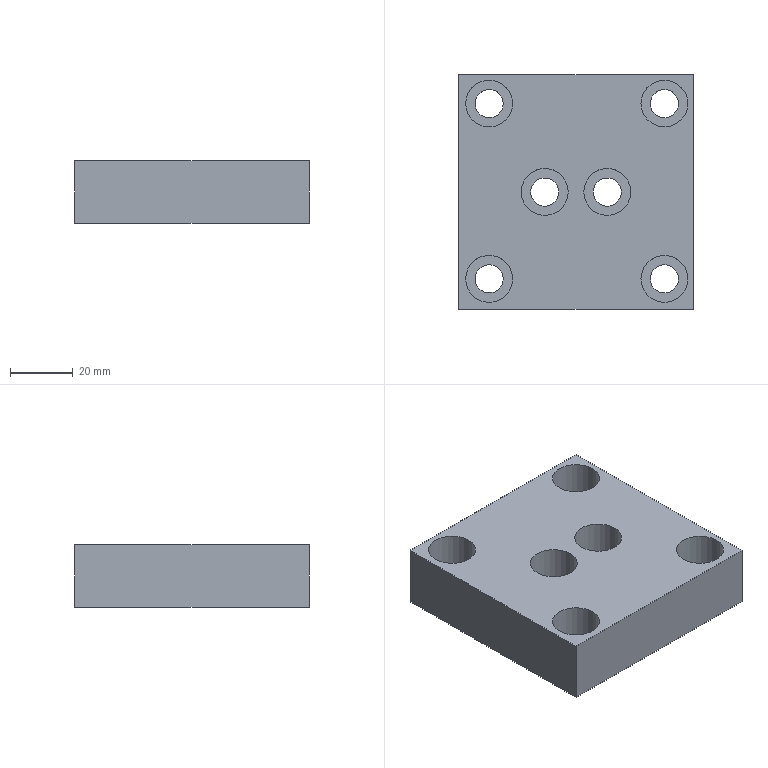Part | NX | features solid 2 | 1 solid | 24 faces | box 75 x 75 x 20 mm | volume 96271 mm3 | plane 12 | cylinder 12 | commonest cylinder face diameters 9 x6 15 x6
STEP:
#1=CARTESIAN_POINT('',(577.5,-142.5,340.));
#2=VERTEX_POINT('',#1);
#3=CARTESIAN_POINT('',(652.5,-142.5,340.));
#4=VERTEX_POINT('',#3);
#5=CARTESIAN_POINT('',(577.5,-142.5,340.));
#6=DIRECTION('',(1.,0.,0.));
#7=VECTOR('',#6,1000.);
#8=LINE('',#5,#7);
#9=EDGE_CURVE('',#2,#4,#8,.T.);
#10=ORIENTED_EDGE('',*,*,#9,.T.);
#11=CARTESIAN_POINT('',(652.5,-142.5,320.));
#12=VERTEX_POINT('',#11);
#13=CARTESIAN_POINT('',(652.5,-142.5,320.));
#14=DIRECTION('',(0.,0.,1.));
#15=VECTOR('',#14,1000.);
#16=LINE('',#13,#15);
#17=EDGE_CURVE('',#12,#4,#16,.T.);
#18=ORIENTED_EDGE('',*,*,#17,.F.);
#19=CARTESIAN_POINT('',(577.5,-142.5,320.));
#20=VERTEX_POINT('',#19);
#21=CARTESIAN_POINT('',(577.5,-142.5,320.));
#22=DIRECTION('',(1.,0.,0.));
#23=VECTOR('',#22,1000.);
#24=LINE('',#21,#23);
#25=EDGE_CURVE('',#20,#12,#24,.T.);
#26=ORIENTED_EDGE('',*,*,#25,.F.);
#27=CARTESIAN_POINT('',(577.5,-142.5,320.));
#28=DIRECTION('',(0.,0.,1.));
#29=VECTOR('',#28,1000.);
#30=LINE('',#27,#29);
#31=EDGE_CURVE('',#20,#2,#30,.T.);
#32=ORIENTED_EDGE('',*,*,#31,.T.);
#33=EDGE_LOOP('',(#10,#18,#26,#32));
#34=FACE_BOUND('',#33,.T.);
#35=CARTESIAN_POINT('',(577.5,-142.5,320.));
#36=DIRECTION('',(0.,-1.,0.));
#37=DIRECTION('',(0.,0.,-1.));
#38=AXIS2_PLACEMENT_3D('',#35,#36,#37);
#39=PLANE('',#38);
#40=ADVANCED_FACE('',(#34),#39,.F.);
#41=CARTESIAN_POINT('',(652.5,-217.5,340.));
#42=VERTEX_POINT('',#41);
#43=CARTESIAN_POINT('',(652.5,-217.5,340.));
#44=DIRECTION('',(0.,1.,0.));
#45=VECTOR('',#44,1000.);
#46=LINE('',#43,#45);
#47=EDGE_CURVE('',#42,#4,#46,.T.);
#48=ORIENTED_EDGE('',*,*,#47,.F.);
#49=CARTESIAN_POINT('',(652.5,-217.5,320.));
#50=VERTEX_POINT('',#49);
#51=CARTESIAN_POINT('',(652.5,-217.5,320.));
#52=DIRECTION('',(0.,0.,1.));
#53=VECTOR('',#52,1000.);
#54=LINE('',#51,#53);
#55=EDGE_CURVE('',#50,#42,#54,.T.);
#56=ORIENTED_EDGE('',*,*,#55,.F.);
#57=CARTESIAN_POINT('',(652.5,-217.5,320.));
#58=DIRECTION('',(0.,1.,0.));
#59=VECTOR('',#58,1000.);
#60=LINE('',#57,#59);
#61=EDGE_CURVE('',#50,#12,#60,.T.);
#62=ORIENTED_EDGE('',*,*,#61,.T.);
#63=ORIENTED_EDGE('',*,*,#17,.T.);
#64=EDGE_LOOP('',(#48,#56,#62,#63));
#65=FACE_BOUND('',#64,.T.);
#66=CARTESIAN_POINT('',(652.5,-217.5,320.));
#67=DIRECTION('',(1.,0.,0.));
#68=DIRECTION('',(0.,0.,-1.));
#69=AXIS2_PLACEMENT_3D('',#66,#67,#68);
#70=PLANE('',#69);
#71=ADVANCED_FACE('',(#65),#70,.T.);
#72=CARTESIAN_POINT('',(577.5,-217.5,340.));
#73=VERTEX_POINT('',#72);
#74=CARTESIAN_POINT('',(577.5,-217.5,340.));
#75=DIRECTION('',(1.,0.,0.));
#76=VECTOR('',#75,1000.);
#77=LINE('',#74,#76);
#78=EDGE_CURVE('',#73,#42,#77,.T.);
#79=ORIENTED_EDGE('',*,*,#78,.F.);
#80=CARTESIAN_POINT('',(577.5,-217.5,320.));
#81=VERTEX_POINT('',#80);
#82=CARTESIAN_POINT('',(577.5,-217.5,320.));
#83=DIRECTION('',(0.,0.,1.));
#84=VECTOR('',#83,1000.);
#85=LINE('',#82,#84);
#86=EDGE_CURVE('',#81,#73,#85,.T.);
#87=ORIENTED_EDGE('',*,*,#86,.F.);
#88=CARTESIAN_POINT('',(577.5,-217.5,320.));
#89=DIRECTION('',(1.,0.,0.));
#90=VECTOR('',#89,1000.);
#91=LINE('',#88,#90);
#92=EDGE_CURVE('',#81,#50,#91,.T.);
#93=ORIENTED_EDGE('',*,*,#92,.T.);
#94=ORIENTED_EDGE('',*,*,#55,.T.);
#95=EDGE_LOOP('',(#79,#87,#93,#94));
#96=FACE_BOUND('',#95,.T.);
#97=CARTESIAN_POINT('',(577.5,-217.5,320.));
#98=DIRECTION('',(0.,-1.,0.));
#99=DIRECTION('',(0.,0.,-1.));
#100=AXIS2_PLACEMENT_3D('',#97,#98,#99);
#101=PLANE('',#100);
#102=ADVANCED_FACE('',(#96),#101,.T.);
#103=CARTESIAN_POINT('',(577.5,-217.5,340.));
#104=DIRECTION('',(0.,1.,0.));
#105=VECTOR('',#104,1000.);
#106=LINE('',#103,#105);
#107=EDGE_CURVE('',#73,#2,#106,.T.);
#108=ORIENTED_EDGE('',*,*,#107,.T.);
#109=ORIENTED_EDGE('',*,*,#31,.F.);
#110=CARTESIAN_POINT('',(577.5,-217.5,320.));
#111=DIRECTION('',(0.,1.,0.));
#112=VECTOR('',#111,1000.);
#113=LINE('',#110,#112);
#114=EDGE_CURVE('',#81,#20,#113,.T.);
#115=ORIENTED_EDGE('',*,*,#114,.F.);
#116=ORIENTED_EDGE('',*,*,#86,.T.);
#117=EDGE_LOOP('',(#108,#109,#115,#116));
#118=FACE_BOUND('',#117,.T.);
#119=CARTESIAN_POINT('',(577.5,-217.5,320.));
#120=DIRECTION('',(1.,0.,0.));
#121=DIRECTION('',(0.,0.,-1.));
#122=AXIS2_PLACEMENT_3D('',#119,#120,#121);
#123=PLANE('',#122);
#124=ADVANCED_FACE('',(#118),#123,.F.);
#125=CARTESIAN_POINT('',(638.75,-207.75,320.));
#126=VERTEX_POINT('',#125);
#127=CARTESIAN_POINT('',(643.25,-207.75,320.));
#128=DIRECTION('',(0.,0.,-1.));
#129=DIRECTION('',(-1.,0.,0.));
#130=AXIS2_PLACEMENT_3D('',#127,#128,#129);
#131=CIRCLE('',#130,4.5);
#132=EDGE_CURVE('',#126,#126,#131,.T.);
#133=ORIENTED_EDGE('',*,*,#132,.F.);
#134=EDGE_LOOP('',(#133));
#135=FACE_BOUND('',#134,.T.);
#136=CARTESIAN_POINT('',(582.75,-207.75,320.));
#137=VERTEX_POINT('',#136);
#138=CARTESIAN_POINT('',(587.25,-207.75,320.));
#139=DIRECTION('',(0.,0.,-1.));
#140=DIRECTION('',(-1.,0.,0.));
#141=AXIS2_PLACEMENT_3D('',#138,#139,#140);
#142=CIRCLE('',#141,4.5);
#143=EDGE_CURVE('',#137,#137,#142,.T.);
#144=ORIENTED_EDGE('',*,*,#143,.F.);
#145=EDGE_LOOP('',(#144));
#146=FACE_BOUND('',#145,.T.);
#147=CARTESIAN_POINT('',(582.75,-151.75,320.));
#148=VERTEX_POINT('',#147);
#149=CARTESIAN_POINT('',(587.25,-151.75,320.));
#150=DIRECTION('',(0.,0.,-1.));
#151=DIRECTION('',(-1.,0.,0.));
#152=AXIS2_PLACEMENT_3D('',#149,#150,#151);
#153=CIRCLE('',#152,4.5);
#154=EDGE_CURVE('',#148,#148,#153,.T.);
#155=ORIENTED_EDGE('',*,*,#154,.F.);
#156=EDGE_LOOP('',(#155));
#157=FACE_BOUND('',#156,.T.);
#158=CARTESIAN_POINT('',(638.75,-151.75,320.));
#159=VERTEX_POINT('',#158);
#160=CARTESIAN_POINT('',(643.25,-151.75,320.));
#161=DIRECTION('',(0.,0.,-1.));
#162=DIRECTION('',(-1.,0.,0.));
#163=AXIS2_PLACEMENT_3D('',#160,#161,#162);
#164=CIRCLE('',#163,4.5);
#165=EDGE_CURVE('',#159,#159,#164,.T.);
#166=ORIENTED_EDGE('',*,*,#165,.F.);
#167=EDGE_LOOP('',(#166));
#168=FACE_BOUND('',#167,.T.);
#169=CARTESIAN_POINT('',(600.5,-180.,320.));
#170=VERTEX_POINT('',#169);
#171=CARTESIAN_POINT('',(605.,-180.,320.));
#172=DIRECTION('',(0.,0.,-1.));
#173=DIRECTION('',(-1.,0.,0.));
#174=AXIS2_PLACEMENT_3D('',#171,#172,#173);
#175=CIRCLE('',#174,4.5);
#176=EDGE_CURVE('',#170,#170,#175,.T.);
#177=ORIENTED_EDGE('',*,*,#176,.F.);
#178=EDGE_LOOP('',(#177));
#179=FACE_BOUND('',#178,.T.);
#180=CARTESIAN_POINT('',(620.5,-180.,320.));
#181=VERTEX_POINT('',#180);
#182=CARTESIAN_POINT('',(625.,-180.,320.));
#183=DIRECTION('',(0.,0.,-1.));
#184=DIRECTION('',(-1.,0.,0.));
#185=AXIS2_PLACEMENT_3D('',#182,#183,#184);
#186=CIRCLE('',#185,4.5);
#187=EDGE_CURVE('',#181,#181,#186,.T.);
#188=ORIENTED_EDGE('',*,*,#187,.F.);
#189=EDGE_LOOP('',(#188));
#190=FACE_BOUND('',#189,.T.);
#191=ORIENTED_EDGE('',*,*,#25,.T.);
#192=ORIENTED_EDGE('',*,*,#61,.F.);
#193=ORIENTED_EDGE('',*,*,#92,.F.);
#194=ORIENTED_EDGE('',*,*,#114,.T.);
#195=EDGE_LOOP('',(#191,#192,#193,#194));
#196=FACE_BOUND('',#195,.T.);
#197=CARTESIAN_POINT('',(652.5,-142.5,320.));
#198=DIRECTION('',(0.,0.,1.));
#199=DIRECTION('',(1.,0.,0.));
#200=AXIS2_PLACEMENT_3D('',#197,#198,#199);
#201=PLANE('',#200);
#202=ADVANCED_FACE('',(#135,#146,#157,#168,#179,#190,#196),#201,.F.);
#203=CARTESIAN_POINT('',(635.75,-207.75,340.));
#204=VERTEX_POINT('',#203);
#205=CARTESIAN_POINT('',(643.25,-207.75,340.));
#206=DIRECTION('',(0.,0.,-1.));
#207=DIRECTION('',(-1.,0.,0.));
#208=AXIS2_PLACEMENT_3D('',#205,#206,#207);
#209=CIRCLE('',#208,7.5);
#210=EDGE_CURVE('',#204,#204,#209,.T.);
#211=ORIENTED_EDGE('',*,*,#210,.T.);
#212=EDGE_LOOP('',(#211));
#213=FACE_BOUND('',#212,.T.);
#214=CARTESIAN_POINT('',(579.75,-207.75,340.));
#215=VERTEX_POINT('',#214);
#216=CARTESIAN_POINT('',(587.25,-207.75,340.));
#217=DIRECTION('',(0.,0.,-1.));
#218=DIRECTION('',(-1.,0.,0.));
#219=AXIS2_PLACEMENT_3D('',#216,#217,#218);
#220=CIRCLE('',#219,7.5);
#221=EDGE_CURVE('',#215,#215,#220,.T.);
#222=ORIENTED_EDGE('',*,*,#221,.T.);
#223=EDGE_LOOP('',(#222));
#224=FACE_BOUND('',#223,.T.);
#225=CARTESIAN_POINT('',(579.75,-151.75,340.));
#226=VERTEX_POINT('',#225);
#227=CARTESIAN_POINT('',(587.25,-151.75,340.));
#228=DIRECTION('',(0.,0.,-1.));
#229=DIRECTION('',(-1.,0.,0.));
#230=AXIS2_PLACEMENT_3D('',#227,#228,#229);
#231=CIRCLE('',#230,7.5);
#232=EDGE_CURVE('',#226,#226,#231,.T.);
#233=ORIENTED_EDGE('',*,*,#232,.T.);
#234=EDGE_LOOP('',(#233));
#235=FACE_BOUND('',#234,.T.);
#236=CARTESIAN_POINT('',(635.75,-151.75,340.));
#237=VERTEX_POINT('',#236);
#238=CARTESIAN_POINT('',(643.25,-151.75,340.));
#239=DIRECTION('',(0.,0.,-1.));
#240=DIRECTION('',(-1.,0.,0.));
#241=AXIS2_PLACEMENT_3D('',#238,#239,#240);
#242=CIRCLE('',#241,7.5);
#243=EDGE_CURVE('',#237,#237,#242,.T.);
#244=ORIENTED_EDGE('',*,*,#243,.T.);
#245=EDGE_LOOP('',(#244));
#246=FACE_BOUND('',#245,.T.);
#247=CARTESIAN_POINT('',(597.5,-180.,340.));
#248=VERTEX_POINT('',#247);
#249=CARTESIAN_POINT('',(605.,-180.,340.));
#250=DIRECTION('',(0.,0.,-1.));
#251=DIRECTION('',(-1.,0.,0.));
#252=AXIS2_PLACEMENT_3D('',#249,#250,#251);
#253=CIRCLE('',#252,7.5);
#254=EDGE_CURVE('',#248,#248,#253,.T.);
#255=ORIENTED_EDGE('',*,*,#254,.T.);
#256=EDGE_LOOP('',(#255));
#257=FACE_BOUND('',#256,.T.);
#258=CARTESIAN_POINT('',(617.5,-180.,340.));
#259=VERTEX_POINT('',#258);
#260=CARTESIAN_POINT('',(625.,-180.,340.));
#261=DIRECTION('',(0.,0.,-1.));
#262=DIRECTION('',(-1.,0.,0.));
#263=AXIS2_PLACEMENT_3D('',#260,#261,#262);
#264=CIRCLE('',#263,7.5);
#265=EDGE_CURVE('',#259,#259,#264,.T.);
#266=ORIENTED_EDGE('',*,*,#265,.T.);
#267=EDGE_LOOP('',(#266));
#268=FACE_BOUND('',#267,.T.);
#269=ORIENTED_EDGE('',*,*,#9,.F.);
#270=ORIENTED_EDGE('',*,*,#107,.F.);
#271=ORIENTED_EDGE('',*,*,#78,.T.);
#272=ORIENTED_EDGE('',*,*,#47,.T.);
#273=EDGE_LOOP('',(#269,#270,#271,#272));
#274=FACE_BOUND('',#273,.T.);
#275=CARTESIAN_POINT('',(652.5,-142.5,340.));
#276=DIRECTION('',(0.,0.,1.));
#277=DIRECTION('',(1.,0.,0.));
#278=AXIS2_PLACEMENT_3D('',#275,#276,#277);
#279=PLANE('',#278);
#280=ADVANCED_FACE('',(#213,#224,#235,#246,#257,#268,#274),#279,.T.);
#281=ORIENTED_EDGE('',*,*,#187,.T.);
#282=EDGE_LOOP('',(#281));
#283=FACE_BOUND('',#282,.T.);
#284=CARTESIAN_POINT('',(620.5,-180.,326.));
#285=VERTEX_POINT('',#284);
#286=CARTESIAN_POINT('',(625.,-180.,326.));
#287=DIRECTION('',(0.,0.,-1.));
#288=DIRECTION('',(-1.,0.,0.));
#289=AXIS2_PLACEMENT_3D('',#286,#287,#288);
#290=CIRCLE('',#289,4.5);
#291=EDGE_CURVE('',#285,#285,#290,.T.);
#292=ORIENTED_EDGE('',*,*,#291,.F.);
#293=EDGE_LOOP('',(#292));
#294=FACE_BOUND('',#293,.T.);
#295=CARTESIAN_POINT('',(625.,-180.,320.));
#296=DIRECTION('',(0.,0.,-1.));
#297=DIRECTION('',(-1.,0.,0.));
#298=AXIS2_PLACEMENT_3D('',#295,#296,#297);
#299=CYLINDRICAL_SURFACE('',#298,4.5);
#300=ADVANCED_FACE('',(#283,#294),#299,.F.);
#301=ORIENTED_EDGE('',*,*,#291,.T.);
#302=EDGE_LOOP('',(#301));
#303=FACE_BOUND('',#302,.T.);
#304=CARTESIAN_POINT('',(617.5,-180.,326.));
#305=VERTEX_POINT('',#304);
#306=CARTESIAN_POINT('',(625.,-180.,326.));
#307=DIRECTION('',(0.,0.,-1.));
#308=DIRECTION('',(-1.,0.,0.));
#309=AXIS2_PLACEMENT_3D('',#306,#307,#308);
#310=CIRCLE('',#309,7.5);
#311=EDGE_CURVE('',#305,#305,#310,.T.);
#312=ORIENTED_EDGE('',*,*,#311,.F.);
#313=EDGE_LOOP('',(#312));
#314=FACE_BOUND('',#313,.T.);
#315=CARTESIAN_POINT('',(625.,-180.,326.));
#316=DIRECTION('',(0.,0.,-1.));
#317=DIRECTION('',(-1.,0.,0.));
#318=AXIS2_PLACEMENT_3D('',#315,#316,#317);
#319=PLANE('',#318);
#320=ADVANCED_FACE('',(#303,#314),#319,.F.);
#321=ORIENTED_EDGE('',*,*,#311,.T.);
#322=EDGE_LOOP('',(#321));
#323=FACE_BOUND('',#322,.T.);
#324=ORIENTED_EDGE('',*,*,#265,.F.);
#325=EDGE_LOOP('',(#324));
#326=FACE_BOUND('',#325,.T.);
#327=CARTESIAN_POINT('',(625.,-180.,340.));
#328=DIRECTION('',(0.,0.,-1.));
#329=DIRECTION('',(-1.,0.,0.));
#330=AXIS2_PLACEMENT_3D('',#327,#328,#329);
#331=CYLINDRICAL_SURFACE('',#330,7.5);
#332=ADVANCED_FACE('',(#323,#326),#331,.F.);
#333=ORIENTED_EDGE('',*,*,#176,.T.);
#334=EDGE_LOOP('',(#333));
#335=FACE_BOUND('',#334,.T.);
#336=CARTESIAN_POINT('',(600.5,-180.,326.));
#337=VERTEX_POINT('',#336);
#338=CARTESIAN_POINT('',(605.,-180.,326.));
#339=DIRECTION('',(0.,0.,-1.));
#340=DIRECTION('',(-1.,0.,0.));
#341=AXIS2_PLACEMENT_3D('',#338,#339,#340);
#342=CIRCLE('',#341,4.5);
#343=EDGE_CURVE('',#337,#337,#342,.T.);
#344=ORIENTED_EDGE('',*,*,#343,.F.);
#345=EDGE_LOOP('',(#344));
#346=FACE_BOUND('',#345,.T.);
#347=CARTESIAN_POINT('',(605.,-180.,320.));
#348=DIRECTION('',(0.,0.,-1.));
#349=DIRECTION('',(-1.,0.,0.));
#350=AXIS2_PLACEMENT_3D('',#347,#348,#349);
#351=CYLINDRICAL_SURFACE('',#350,4.5);
#352=ADVANCED_FACE('',(#335,#346),#351,.F.);
#353=ORIENTED_EDGE('',*,*,#343,.T.);
#354=EDGE_LOOP('',(#353));
#355=FACE_BOUND('',#354,.T.);
#356=CARTESIAN_POINT('',(597.5,-180.,326.));
#357=VERTEX_POINT('',#356);
#358=CARTESIAN_POINT('',(605.,-180.,326.));
#359=DIRECTION('',(0.,0.,-1.));
#360=DIRECTION('',(-1.,0.,0.));
#361=AXIS2_PLACEMENT_3D('',#358,#359,#360);
#362=CIRCLE('',#361,7.5);
#363=EDGE_CURVE('',#357,#357,#362,.T.);
#364=ORIENTED_EDGE('',*,*,#363,.F.);
#365=EDGE_LOOP('',(#364));
#366=FACE_BOUND('',#365,.T.);
#367=CARTESIAN_POINT('',(605.,-180.,326.));
#368=DIRECTION('',(0.,0.,-1.));
#369=DIRECTION('',(-1.,0.,0.));
#370=AXIS2_PLACEMENT_3D('',#367,#368,#369);
#371=PLANE('',#370);
#372=ADVANCED_FACE('',(#355,#366),#371,.F.);
#373=ORIENTED_EDGE('',*,*,#363,.T.);
#374=EDGE_LOOP('',(#373));
#375=FACE_BOUND('',#374,.T.);
#376=ORIENTED_EDGE('',*,*,#254,.F.);
#377=EDGE_LOOP('',(#376));
#378=FACE_BOUND('',#377,.T.);
#379=CARTESIAN_POINT('',(605.,-180.,340.));
#380=DIRECTION('',(0.,0.,-1.));
#381=DIRECTION('',(-1.,0.,0.));
#382=AXIS2_PLACEMENT_3D('',#379,#380,#381);
#383=CYLINDRICAL_SURFACE('',#382,7.5);
#384=ADVANCED_FACE('',(#375,#378),#383,.F.);
#385=ORIENTED_EDGE('',*,*,#165,.T.);
#386=EDGE_LOOP('',(#385));
#387=FACE_BOUND('',#386,.T.);
#388=CARTESIAN_POINT('',(638.75,-151.75,328.));
#389=VERTEX_POINT('',#388);
#390=CARTESIAN_POINT('',(643.25,-151.75,328.));
#391=DIRECTION('',(0.,0.,-1.));
#392=DIRECTION('',(-1.,0.,0.));
#393=AXIS2_PLACEMENT_3D('',#390,#391,#392);
#394=CIRCLE('',#393,4.5);
#395=EDGE_CURVE('',#389,#389,#394,.T.);
#396=ORIENTED_EDGE('',*,*,#395,.F.);
#397=EDGE_LOOP('',(#396));
#398=FACE_BOUND('',#397,.T.);
#399=CARTESIAN_POINT('',(643.25,-151.75,320.));
#400=DIRECTION('',(0.,0.,-1.));
#401=DIRECTION('',(-1.,0.,0.));
#402=AXIS2_PLACEMENT_3D('',#399,#400,#401);
#403=CYLINDRICAL_SURFACE('',#402,4.5);
#404=ADVANCED_FACE('',(#387,#398),#403,.F.);
#405=ORIENTED_EDGE('',*,*,#395,.T.);
#406=EDGE_LOOP('',(#405));
#407=FACE_BOUND('',#406,.T.);
#408=CARTESIAN_POINT('',(635.75,-151.75,328.));
#409=VERTEX_POINT('',#408);
#410=CARTESIAN_POINT('',(643.25,-151.75,328.));
#411=DIRECTION('',(0.,0.,-1.));
#412=DIRECTION('',(-1.,0.,0.));
#413=AXIS2_PLACEMENT_3D('',#410,#411,#412);
#414=CIRCLE('',#413,7.5);
#415=EDGE_CURVE('',#409,#409,#414,.T.);
#416=ORIENTED_EDGE('',*,*,#415,.F.);
#417=EDGE_LOOP('',(#416));
#418=FACE_BOUND('',#417,.T.);
#419=CARTESIAN_POINT('',(643.25,-151.75,328.));
#420=DIRECTION('',(0.,0.,-1.));
#421=DIRECTION('',(-1.,0.,0.));
#422=AXIS2_PLACEMENT_3D('',#419,#420,#421);
#423=PLANE('',#422);
#424=ADVANCED_FACE('',(#407,#418),#423,.F.);
#425=ORIENTED_EDGE('',*,*,#415,.T.);
#426=EDGE_LOOP('',(#425));
#427=FACE_BOUND('',#426,.T.);
#428=ORIENTED_EDGE('',*,*,#243,.F.);
#429=EDGE_LOOP('',(#428));
#430=FACE_BOUND('',#429,.T.);
#431=CARTESIAN_POINT('',(643.25,-151.75,340.));
#432=DIRECTION('',(0.,0.,-1.));
#433=DIRECTION('',(-1.,0.,0.));
#434=AXIS2_PLACEMENT_3D('',#431,#432,#433);
#435=CYLINDRICAL_SURFACE('',#434,7.5);
#436=ADVANCED_FACE('',(#427,#430),#435,.F.);
#437=ORIENTED_EDGE('',*,*,#154,.T.);
#438=EDGE_LOOP('',(#437));
#439=FACE_BOUND('',#438,.T.);
#440=CARTESIAN_POINT('',(582.75,-151.75,328.));
#441=VERTEX_POINT('',#440);
#442=CARTESIAN_POINT('',(587.25,-151.75,328.));
#443=DIRECTION('',(0.,0.,-1.));
#444=DIRECTION('',(-1.,0.,0.));
#445=AXIS2_PLACEMENT_3D('',#442,#443,#444);
#446=CIRCLE('',#445,4.5);
#447=EDGE_CURVE('',#441,#441,#446,.T.);
#448=ORIENTED_EDGE('',*,*,#447,.F.);
#449=EDGE_LOOP('',(#448));
#450=FACE_BOUND('',#449,.T.);
#451=CARTESIAN_POINT('',(587.25,-151.75,320.));
#452=DIRECTION('',(0.,0.,-1.));
#453=DIRECTION('',(-1.,0.,0.));
#454=AXIS2_PLACEMENT_3D('',#451,#452,#453);
#455=CYLINDRICAL_SURFACE('',#454,4.5);
#456=ADVANCED_FACE('',(#439,#450),#455,.F.);
#457=ORIENTED_EDGE('',*,*,#447,.T.);
#458=EDGE_LOOP('',(#457));
#459=FACE_BOUND('',#458,.T.);
#460=CARTESIAN_POINT('',(579.75,-151.75,328.));
#461=VERTEX_POINT('',#460);
#462=CARTESIAN_POINT('',(587.25,-151.75,328.));
#463=DIRECTION('',(0.,0.,-1.));
#464=DIRECTION('',(-1.,0.,0.));
#465=AXIS2_PLACEMENT_3D('',#462,#463,#464);
#466=CIRCLE('',#465,7.5);
#467=EDGE_CURVE('',#461,#461,#466,.T.);
#468=ORIENTED_EDGE('',*,*,#467,.F.);
#469=EDGE_LOOP('',(#468));
#470=FACE_BOUND('',#469,.T.);
#471=CARTESIAN_POINT('',(587.25,-151.75,328.));
#472=DIRECTION('',(0.,0.,-1.));
#473=DIRECTION('',(-1.,0.,0.));
#474=AXIS2_PLACEMENT_3D('',#471,#472,#473);
#475=PLANE('',#474);
#476=ADVANCED_FACE('',(#459,#470),#475,.F.);
#477=ORIENTED_EDGE('',*,*,#467,.T.);
#478=EDGE_LOOP('',(#477));
#479=FACE_BOUND('',#478,.T.);
#480=ORIENTED_EDGE('',*,*,#232,.F.);
#481=EDGE_LOOP('',(#480));
#482=FACE_BOUND('',#481,.T.);
#483=CARTESIAN_POINT('',(587.25,-151.75,340.));
#484=DIRECTION('',(0.,0.,-1.));
#485=DIRECTION('',(-1.,0.,0.));
#486=AXIS2_PLACEMENT_3D('',#483,#484,#485);
#487=CYLINDRICAL_SURFACE('',#486,7.5);
#488=ADVANCED_FACE('',(#479,#482),#487,.F.);
#489=ORIENTED_EDGE('',*,*,#143,.T.);
#490=EDGE_LOOP('',(#489));
#491=FACE_BOUND('',#490,.T.);
#492=CARTESIAN_POINT('',(582.75,-207.75,328.));
#493=VERTEX_POINT('',#492);
#494=CARTESIAN_POINT('',(587.25,-207.75,328.));
#495=DIRECTION('',(0.,0.,-1.));
#496=DIRECTION('',(-1.,0.,0.));
#497=AXIS2_PLACEMENT_3D('',#494,#495,#496);
#498=CIRCLE('',#497,4.5);
#499=EDGE_CURVE('',#493,#493,#498,.T.);
#500=ORIENTED_EDGE('',*,*,#499,.F.);
#501=EDGE_LOOP('',(#500));
#502=FACE_BOUND('',#501,.T.);
#503=CARTESIAN_POINT('',(587.25,-207.75,320.));
#504=DIRECTION('',(0.,0.,-1.));
#505=DIRECTION('',(-1.,0.,0.));
#506=AXIS2_PLACEMENT_3D('',#503,#504,#505);
#507=CYLINDRICAL_SURFACE('',#506,4.5);
#508=ADVANCED_FACE('',(#491,#502),#507,.F.);
#509=ORIENTED_EDGE('',*,*,#499,.T.);
#510=EDGE_LOOP('',(#509));
#511=FACE_BOUND('',#510,.T.);
#512=CARTESIAN_POINT('',(579.75,-207.75,328.));
#513=VERTEX_POINT('',#512);
#514=CARTESIAN_POINT('',(587.25,-207.75,328.));
#515=DIRECTION('',(0.,0.,-1.));
#516=DIRECTION('',(-1.,0.,0.));
#517=AXIS2_PLACEMENT_3D('',#514,#515,#516);
#518=CIRCLE('',#517,7.5);
#519=EDGE_CURVE('',#513,#513,#518,.T.);
#520=ORIENTED_EDGE('',*,*,#519,.F.);
#521=EDGE_LOOP('',(#520));
#522=FACE_BOUND('',#521,.T.);
#523=CARTESIAN_POINT('',(587.25,-207.75,328.));
#524=DIRECTION('',(0.,0.,-1.));
#525=DIRECTION('',(-1.,0.,0.));
#526=AXIS2_PLACEMENT_3D('',#523,#524,#525);
#527=PLANE('',#526);
#528=ADVANCED_FACE('',(#511,#522),#527,.F.);
#529=ORIENTED_EDGE('',*,*,#519,.T.);
#530=EDGE_LOOP('',(#529));
#531=FACE_BOUND('',#530,.T.);
#532=ORIENTED_EDGE('',*,*,#221,.F.);
#533=EDGE_LOOP('',(#532));
#534=FACE_BOUND('',#533,.T.);
#535=CARTESIAN_POINT('',(587.25,-207.75,340.));
#536=DIRECTION('',(0.,0.,-1.));
#537=DIRECTION('',(-1.,0.,0.));
#538=AXIS2_PLACEMENT_3D('',#535,#536,#537);
#539=CYLINDRICAL_SURFACE('',#538,7.5);
#540=ADVANCED_FACE('',(#531,#534),#539,.F.);
#541=ORIENTED_EDGE('',*,*,#132,.T.);
#542=EDGE_LOOP('',(#541));
#543=FACE_BOUND('',#542,.T.);
#544=CARTESIAN_POINT('',(638.75,-207.75,328.));
#545=VERTEX_POINT('',#544);
#546=CARTESIAN_POINT('',(643.25,-207.75,328.));
#547=DIRECTION('',(0.,0.,-1.));
#548=DIRECTION('',(-1.,0.,0.));
#549=AXIS2_PLACEMENT_3D('',#546,#547,#548);
#550=CIRCLE('',#549,4.5);
#551=EDGE_CURVE('',#545,#545,#550,.T.);
#552=ORIENTED_EDGE('',*,*,#551,.F.);
#553=EDGE_LOOP('',(#552));
#554=FACE_BOUND('',#553,.T.);
#555=CARTESIAN_POINT('',(643.25,-207.75,320.));
#556=DIRECTION('',(0.,0.,-1.));
#557=DIRECTION('',(-1.,0.,0.));
#558=AXIS2_PLACEMENT_3D('',#555,#556,#557);
#559=CYLINDRICAL_SURFACE('',#558,4.5);
#560=ADVANCED_FACE('',(#543,#554),#559,.F.);
#561=ORIENTED_EDGE('',*,*,#551,.T.);
#562=EDGE_LOOP('',(#561));
#563=FACE_BOUND('',#562,.T.);
#564=CARTESIAN_POINT('',(635.75,-207.75,328.));
#565=VERTEX_POINT('',#564);
#566=CARTESIAN_POINT('',(643.25,-207.75,328.));
#567=DIRECTION('',(0.,0.,-1.));
#568=DIRECTION('',(-1.,0.,0.));
#569=AXIS2_PLACEMENT_3D('',#566,#567,#568);
#570=CIRCLE('',#569,7.5);
#571=EDGE_CURVE('',#565,#565,#570,.T.);
#572=ORIENTED_EDGE('',*,*,#571,.F.);
#573=EDGE_LOOP('',(#572));
#574=FACE_BOUND('',#573,.T.);
#575=CARTESIAN_POINT('',(643.25,-207.75,328.));
#576=DIRECTION('',(0.,0.,-1.));
#577=DIRECTION('',(-1.,0.,0.));
#578=AXIS2_PLACEMENT_3D('',#575,#576,#577);
#579=PLANE('',#578);
#580=ADVANCED_FACE('',(#563,#574),#579,.F.);
#581=ORIENTED_EDGE('',*,*,#571,.T.);
#582=EDGE_LOOP('',(#581));
#583=FACE_BOUND('',#582,.T.);
#584=ORIENTED_EDGE('',*,*,#210,.F.);
#585=EDGE_LOOP('',(#584));
#586=FACE_BOUND('',#585,.T.);
#587=CARTESIAN_POINT('',(643.25,-207.75,340.));
#588=DIRECTION('',(0.,0.,-1.));
#589=DIRECTION('',(-1.,0.,0.));
#590=AXIS2_PLACEMENT_3D('',#587,#588,#589);
#591=CYLINDRICAL_SURFACE('',#590,7.5);
#592=ADVANCED_FACE('',(#583,#586),#591,.F.);
#593=CLOSED_SHELL('',(#40,#71,#102,#124,#202,#280,#300,#320,#332,#352,#372,#384,#404,#424,#436,#456,#476,#488,#508,#528,#540,#560,#580,#592));
#594=MANIFOLD_SOLID_BREP('',#593);
#595=(LENGTH_UNIT()NAMED_UNIT(*)SI_UNIT(.MILLI.,.METRE.));
#596=UNCERTAINTY_MEASURE_WITH_UNIT(LENGTH_MEASURE(0.00001),#595,'','');
#597=(NAMED_UNIT(*)PLANE_ANGLE_UNIT()SI_UNIT($,.RADIAN.));
#598=(NAMED_UNIT(*)SI_UNIT($,.STERADIAN.)SOLID_ANGLE_UNIT());
#599=(GEOMETRIC_REPRESENTATION_CONTEXT(3)GLOBAL_UNCERTAINTY_ASSIGNED_CONTEXT((#596))GLOBAL_UNIT_ASSIGNED_CONTEXT((#595,#597,#598))REPRESENTATION_CONTEXT('',''));
#600=ADVANCED_BREP_SHAPE_REPRESENTATION('',(#594),#599);